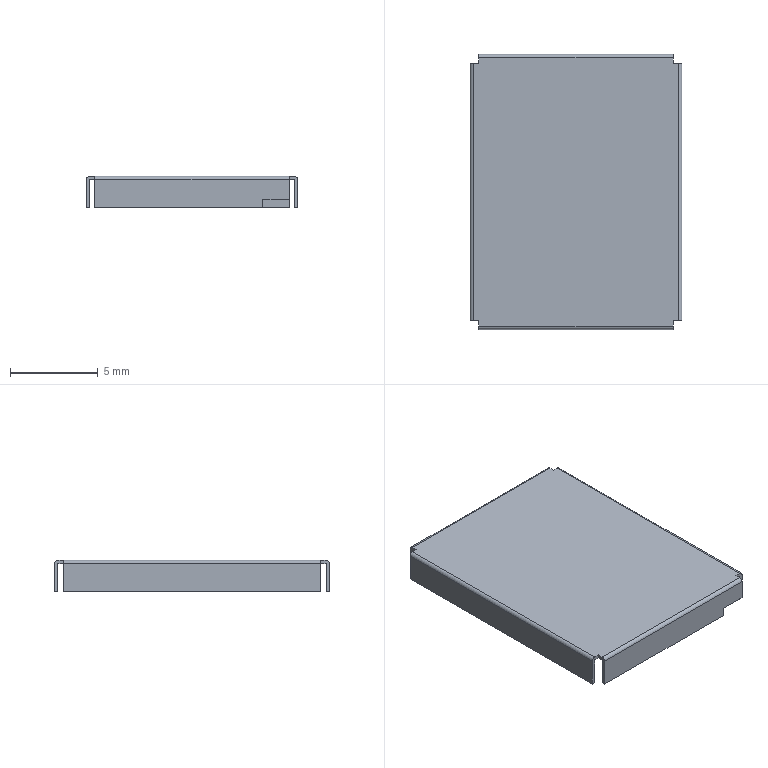Part | Creo | 1 solid | 28 faces | box 12.1 x 15.71 x 1.8 mm | volume 53.743 mm3 | plane 24 | cylinder 4 | commonest cylinder face diameters 0.4 x4
STEP:
#1=CARTESIAN_POINT('',(0.,0.,0.));
#2=DIRECTION('',(0.,0.,1.));
#3=DIRECTION('',(1.,0.,0.));
#4=AXIS2_PLACEMENT_3D('',#1,#2,#3);
#5=CARTESIAN_POINT('',(-0.1,15.11,0.));
#6=VERTEX_POINT('',#5);
#7=CARTESIAN_POINT('',(0.1,15.11,0.));
#8=VERTEX_POINT('',#7);
#9=CARTESIAN_POINT('',(-0.1,15.11,0.));
#10=DIRECTION('',(1.,0.,0.));
#11=VECTOR('',#10,0.2);
#12=LINE('',#9,#11);
#13=EDGE_CURVE('',#6,#8,#12,.T.);
#14=ORIENTED_EDGE('',*,*,#13,.F.);
#15=CARTESIAN_POINT('',(-0.1,0.4,0.));
#16=VERTEX_POINT('',#15);
#17=CARTESIAN_POINT('',(-0.1,15.11,0.));
#18=DIRECTION('',(0.,-1.,0.));
#19=VECTOR('',#18,14.71);
#20=LINE('',#17,#19);
#21=EDGE_CURVE('',#6,#16,#20,.T.);
#22=ORIENTED_EDGE('',*,*,#21,.T.);
#23=CARTESIAN_POINT('',(0.1,0.4,0.));
#24=VERTEX_POINT('',#23);
#25=CARTESIAN_POINT('',(-0.1,0.4,0.));
#26=DIRECTION('',(1.,0.,0.));
#27=VECTOR('',#26,0.2);
#28=LINE('',#25,#27);
#29=EDGE_CURVE('',#16,#24,#28,.T.);
#30=ORIENTED_EDGE('',*,*,#29,.T.);
#31=CARTESIAN_POINT('',(0.1,15.11,0.));
#32=DIRECTION('',(0.,-1.,0.));
#33=VECTOR('',#32,14.71);
#34=LINE('',#31,#33);
#35=EDGE_CURVE('',#8,#24,#34,.T.);
#36=ORIENTED_EDGE('',*,*,#35,.F.);
#37=EDGE_LOOP('',(#14,#22,#30,#36));
#38=FACE_OUTER_BOUND('',#37,.F.);
#39=CARTESIAN_POINT('',(0.,0.,0.));
#40=DIRECTION('',(0.,0.,1.));
#41=DIRECTION('',(1.,0.,0.));
#42=AXIS2_PLACEMENT_3D('',#39,#40,#41);
#43=PLANE('',#42);
#44=ADVANCED_FACE('',(#38),#43,.F.);
#45=ORIENTED_EDGE('',*,*,#13,.T.);
#46=CARTESIAN_POINT('',(0.1,15.11,1.6));
#47=VERTEX_POINT('',#46);
#48=CARTESIAN_POINT('',(0.1,15.11,0.));
#49=DIRECTION('',(0.,0.,1.));
#50=VECTOR('',#49,1.6);
#51=LINE('',#48,#50);
#52=EDGE_CURVE('',#8,#47,#51,.T.);
#53=ORIENTED_EDGE('',*,*,#52,.T.);
#54=CARTESIAN_POINT('',(0.4,15.11,1.6));
#55=VERTEX_POINT('',#54);
#56=CARTESIAN_POINT('',(0.1,15.11,1.6));
#57=DIRECTION('',(1.,0.,0.));
#58=VECTOR('',#57,0.3);
#59=LINE('',#56,#58);
#60=EDGE_CURVE('',#47,#55,#59,.T.);
#61=ORIENTED_EDGE('',*,*,#60,.T.);
#62=CARTESIAN_POINT('',(0.4,15.11,1.8));
#63=VERTEX_POINT('',#62);
#64=CARTESIAN_POINT('',(0.4,15.11,1.8));
#65=DIRECTION('',(0.,0.,-1.));
#66=VECTOR('',#65,0.2);
#67=LINE('',#64,#66);
#68=EDGE_CURVE('',#63,#55,#67,.T.);
#69=ORIENTED_EDGE('',*,*,#68,.F.);
#70=CARTESIAN_POINT('',(0.1,15.11,1.8));
#71=VERTEX_POINT('',#70);
#72=CARTESIAN_POINT('',(0.1,15.11,1.8));
#73=DIRECTION('',(1.,0.,0.));
#74=VECTOR('',#73,0.3);
#75=LINE('',#72,#74);
#76=EDGE_CURVE('',#71,#63,#75,.T.);
#77=ORIENTED_EDGE('',*,*,#76,.F.);
#78=CARTESIAN_POINT('',(-0.1,15.11,1.6));
#79=VERTEX_POINT('',#78);
#80=CARTESIAN_POINT('',(0.1,15.11,1.6));
#81=DIRECTION('',(0.,-1.,0.));
#82=DIRECTION('',(0.,0.,1.));
#83=AXIS2_PLACEMENT_3D('',#80,#81,#82);
#84=CIRCLE('',#83,0.2);
#85=EDGE_CURVE('',#71,#79,#84,.T.);
#86=ORIENTED_EDGE('',*,*,#85,.T.);
#87=CARTESIAN_POINT('',(-0.1,15.11,0.));
#88=DIRECTION('',(0.,0.,1.));
#89=VECTOR('',#88,1.6);
#90=LINE('',#87,#89);
#91=EDGE_CURVE('',#6,#79,#90,.T.);
#92=ORIENTED_EDGE('',*,*,#91,.F.);
#93=EDGE_LOOP('',(#45,#53,#61,#69,#77,#86,#92));
#94=FACE_OUTER_BOUND('',#93,.F.);
#95=CARTESIAN_POINT('',(-0.1,15.11,1.8));
#96=DIRECTION('',(0.,-1.,0.));
#97=DIRECTION('',(1.,0.,0.));
#98=AXIS2_PLACEMENT_3D('',#95,#96,#97);
#99=PLANE('',#98);
#100=ADVANCED_FACE('',(#94),#99,.F.);
#101=ORIENTED_EDGE('',*,*,#52,.F.);
#102=ORIENTED_EDGE('',*,*,#35,.T.);
#103=CARTESIAN_POINT('',(0.1,0.4,1.6));
#104=VERTEX_POINT('',#103);
#105=CARTESIAN_POINT('',(0.1,0.4,0.));
#106=DIRECTION('',(0.,0.,1.));
#107=VECTOR('',#106,1.6);
#108=LINE('',#105,#107);
#109=EDGE_CURVE('',#24,#104,#108,.T.);
#110=ORIENTED_EDGE('',*,*,#109,.T.);
#111=CARTESIAN_POINT('',(0.1,15.11,1.6));
#112=DIRECTION('',(0.,-1.,0.));
#113=VECTOR('',#112,14.71);
#114=LINE('',#111,#113);
#115=EDGE_CURVE('',#47,#104,#114,.T.);
#116=ORIENTED_EDGE('',*,*,#115,.F.);
#117=EDGE_LOOP('',(#101,#102,#110,#116));
#118=FACE_OUTER_BOUND('',#117,.F.);
#119=CARTESIAN_POINT('',(0.1,15.61,0.));
#120=DIRECTION('',(-1.,0.,0.));
#121=DIRECTION('',(0.,-1.,0.));
#122=AXIS2_PLACEMENT_3D('',#119,#120,#121);
#123=PLANE('',#122);
#124=ADVANCED_FACE('',(#118),#123,.F.);
#125=ORIENTED_EDGE('',*,*,#29,.F.);
#126=CARTESIAN_POINT('',(-0.1,0.4,1.6));
#127=VERTEX_POINT('',#126);
#128=CARTESIAN_POINT('',(-0.1,0.4,0.));
#129=DIRECTION('',(0.,0.,1.));
#130=VECTOR('',#129,1.6);
#131=LINE('',#128,#130);
#132=EDGE_CURVE('',#16,#127,#131,.T.);
#133=ORIENTED_EDGE('',*,*,#132,.T.);
#134=CARTESIAN_POINT('',(0.1,0.4,1.8));
#135=VERTEX_POINT('',#134);
#136=CARTESIAN_POINT('',(0.1,0.4,1.6));
#137=DIRECTION('',(0.,1.,0.));
#138=DIRECTION('',(-1.,0.,0.));
#139=AXIS2_PLACEMENT_3D('',#136,#137,#138);
#140=CIRCLE('',#139,0.2);
#141=EDGE_CURVE('',#127,#135,#140,.T.);
#142=ORIENTED_EDGE('',*,*,#141,.T.);
#143=CARTESIAN_POINT('',(0.4,0.4,1.8));
#144=VERTEX_POINT('',#143);
#145=CARTESIAN_POINT('',(0.1,0.4,1.8));
#146=DIRECTION('',(1.,0.,0.));
#147=VECTOR('',#146,0.3);
#148=LINE('',#145,#147);
#149=EDGE_CURVE('',#135,#144,#148,.T.);
#150=ORIENTED_EDGE('',*,*,#149,.T.);
#151=CARTESIAN_POINT('',(0.4,0.4,1.6));
#152=VERTEX_POINT('',#151);
#153=CARTESIAN_POINT('',(0.4,0.4,1.8));
#154=DIRECTION('',(0.,0.,-1.));
#155=VECTOR('',#154,0.2);
#156=LINE('',#153,#155);
#157=EDGE_CURVE('',#144,#152,#156,.T.);
#158=ORIENTED_EDGE('',*,*,#157,.T.);
#159=CARTESIAN_POINT('',(0.1,0.4,1.6));
#160=DIRECTION('',(1.,0.,0.));
#161=VECTOR('',#160,0.3);
#162=LINE('',#159,#161);
#163=EDGE_CURVE('',#104,#152,#162,.T.);
#164=ORIENTED_EDGE('',*,*,#163,.F.);
#165=ORIENTED_EDGE('',*,*,#109,.F.);
#166=EDGE_LOOP('',(#125,#133,#142,#150,#158,#164,#165));
#167=FACE_OUTER_BOUND('',#166,.F.);
#168=CARTESIAN_POINT('',(0.4,0.4,1.8));
#169=DIRECTION('',(0.,1.,0.));
#170=DIRECTION('',(-1.,0.,0.));
#171=AXIS2_PLACEMENT_3D('',#168,#169,#170);
#172=PLANE('',#171);
#173=ADVANCED_FACE('',(#167),#172,.F.);
#174=ORIENTED_EDGE('',*,*,#91,.T.);
#175=CARTESIAN_POINT('',(-0.1,0.4,1.6));
#176=DIRECTION('',(0.,1.,0.));
#177=VECTOR('',#176,14.71);
#178=LINE('',#175,#177);
#179=EDGE_CURVE('',#127,#79,#178,.T.);
#180=ORIENTED_EDGE('',*,*,#179,.F.);
#181=ORIENTED_EDGE('',*,*,#132,.F.);
#182=ORIENTED_EDGE('',*,*,#21,.F.);
#183=EDGE_LOOP('',(#174,#180,#181,#182));
#184=FACE_OUTER_BOUND('',#183,.F.);
#185=CARTESIAN_POINT('',(-0.1,15.61,0.));
#186=DIRECTION('',(-1.,0.,0.));
#187=DIRECTION('',(0.,-1.,0.));
#188=AXIS2_PLACEMENT_3D('',#185,#186,#187);
#189=PLANE('',#188);
#190=ADVANCED_FACE('',(#184),#189,.T.);
#191=ORIENTED_EDGE('',*,*,#85,.F.);
#192=CARTESIAN_POINT('',(0.1,15.11,1.8));
#193=DIRECTION('',(0.,-1.,0.));
#194=VECTOR('',#193,14.71);
#195=LINE('',#192,#194);
#196=EDGE_CURVE('',#71,#135,#195,.T.);
#197=ORIENTED_EDGE('',*,*,#196,.T.);
#198=ORIENTED_EDGE('',*,*,#141,.F.);
#199=ORIENTED_EDGE('',*,*,#179,.T.);
#200=EDGE_LOOP('',(#191,#197,#198,#199));
#201=FACE_OUTER_BOUND('',#200,.F.);
#202=CARTESIAN_POINT('',(0.1,36.247,1.6));
#203=DIRECTION('',(0.,-1.,0.));
#204=DIRECTION('',(0.,0.,1.));
#205=AXIS2_PLACEMENT_3D('',#202,#203,#204);
#206=CYLINDRICAL_SURFACE('',#205,0.2);
#207=ADVANCED_FACE('',(#201),#206,.T.);
#208=ORIENTED_EDGE('',*,*,#76,.T.);
#209=CARTESIAN_POINT('',(0.4,15.41,1.8));
#210=VERTEX_POINT('',#209);
#211=CARTESIAN_POINT('',(0.4,15.41,1.8));
#212=DIRECTION('',(0.,-1.,0.));
#213=VECTOR('',#212,0.3);
#214=LINE('',#211,#213);
#215=EDGE_CURVE('',#210,#63,#214,.T.);
#216=ORIENTED_EDGE('',*,*,#215,.F.);
#217=CARTESIAN_POINT('',(11.5,15.41,1.8));
#218=VERTEX_POINT('',#217);
#219=CARTESIAN_POINT('',(11.5,15.41,1.8));
#220=DIRECTION('',(-1.,0.,0.));
#221=VECTOR('',#220,11.1);
#222=LINE('',#219,#221);
#223=EDGE_CURVE('',#218,#210,#222,.T.);
#224=ORIENTED_EDGE('',*,*,#223,.F.);
#225=CARTESIAN_POINT('',(11.5,15.11,1.8));
#226=VERTEX_POINT('',#225);
#227=CARTESIAN_POINT('',(11.5,15.41,1.8));
#228=DIRECTION('',(0.,-1.,0.));
#229=VECTOR('',#228,0.3);
#230=LINE('',#227,#229);
#231=EDGE_CURVE('',#218,#226,#230,.T.);
#232=ORIENTED_EDGE('',*,*,#231,.T.);
#233=CARTESIAN_POINT('',(11.8,15.11,1.8));
#234=VERTEX_POINT('',#233);
#235=CARTESIAN_POINT('',(11.8,15.11,1.8));
#236=DIRECTION('',(-1.,0.,0.));
#237=VECTOR('',#236,0.3);
#238=LINE('',#235,#237);
#239=EDGE_CURVE('',#234,#226,#238,.T.);
#240=ORIENTED_EDGE('',*,*,#239,.F.);
#241=CARTESIAN_POINT('',(11.8,0.4,1.8));
#242=VERTEX_POINT('',#241);
#243=CARTESIAN_POINT('',(11.8,0.4,1.8));
#244=DIRECTION('',(0.,1.,0.));
#245=VECTOR('',#244,14.71);
#246=LINE('',#243,#245);
#247=EDGE_CURVE('',#242,#234,#246,.T.);
#248=ORIENTED_EDGE('',*,*,#247,.F.);
#249=CARTESIAN_POINT('',(11.5,0.4,1.8));
#250=VERTEX_POINT('',#249);
#251=CARTESIAN_POINT('',(11.8,0.4,1.8));
#252=DIRECTION('',(-1.,0.,0.));
#253=VECTOR('',#252,0.3);
#254=LINE('',#251,#253);
#255=EDGE_CURVE('',#242,#250,#254,.T.);
#256=ORIENTED_EDGE('',*,*,#255,.T.);
#257=CARTESIAN_POINT('',(11.5,0.1,1.8));
#258=VERTEX_POINT('',#257);
#259=CARTESIAN_POINT('',(11.5,0.1,1.8));
#260=DIRECTION('',(0.,1.,0.));
#261=VECTOR('',#260,0.3);
#262=LINE('',#259,#261);
#263=EDGE_CURVE('',#258,#250,#262,.T.);
#264=ORIENTED_EDGE('',*,*,#263,.F.);
#265=CARTESIAN_POINT('',(0.4,0.1,1.8));
#266=VERTEX_POINT('',#265);
#267=CARTESIAN_POINT('',(0.4,0.1,1.8));
#268=DIRECTION('',(1.,0.,0.));
#269=VECTOR('',#268,11.1);
#270=LINE('',#267,#269);
#271=EDGE_CURVE('',#266,#258,#270,.T.);
#272=ORIENTED_EDGE('',*,*,#271,.F.);
#273=CARTESIAN_POINT('',(0.4,0.1,1.8));
#274=DIRECTION('',(0.,1.,0.));
#275=VECTOR('',#274,0.3);
#276=LINE('',#273,#275);
#277=EDGE_CURVE('',#266,#144,#276,.T.);
#278=ORIENTED_EDGE('',*,*,#277,.T.);
#279=ORIENTED_EDGE('',*,*,#149,.F.);
#280=ORIENTED_EDGE('',*,*,#196,.F.);
#281=EDGE_LOOP('',(#208,#216,#224,#232,#240,#248,#256,#264,#272,#278,#279,#280));
#282=FACE_OUTER_BOUND('',#281,.F.);
#283=CARTESIAN_POINT('',(0.,0.,1.8));
#284=DIRECTION('',(0.,0.,1.));
#285=DIRECTION('',(1.,0.,0.));
#286=AXIS2_PLACEMENT_3D('',#283,#284,#285);
#287=PLANE('',#286);
#288=ADVANCED_FACE('',(#282),#287,.T.);
#289=CARTESIAN_POINT('',(0.4,15.61,0.));
#290=VERTEX_POINT('',#289);
#291=CARTESIAN_POINT('',(0.4,15.41,0.));
#292=VERTEX_POINT('',#291);
#293=CARTESIAN_POINT('',(0.4,15.61,0.));
#294=DIRECTION('',(0.,-1.,0.));
#295=VECTOR('',#294,0.2);
#296=LINE('',#293,#295);
#297=EDGE_CURVE('',#290,#292,#296,.T.);
#298=ORIENTED_EDGE('',*,*,#297,.F.);
#299=CARTESIAN_POINT('',(0.4,15.61,1.6));
#300=VERTEX_POINT('',#299);
#301=CARTESIAN_POINT('',(0.4,15.61,0.));
#302=DIRECTION('',(0.,0.,1.));
#303=VECTOR('',#302,1.6);
#304=LINE('',#301,#303);
#305=EDGE_CURVE('',#290,#300,#304,.T.);
#306=ORIENTED_EDGE('',*,*,#305,.T.);
#307=CARTESIAN_POINT('',(0.4,15.41,1.6));
#308=DIRECTION('',(1.,0.,0.));
#309=DIRECTION('',(0.,1.,0.));
#310=AXIS2_PLACEMENT_3D('',#307,#308,#309);
#311=CIRCLE('',#310,0.2);
#312=EDGE_CURVE('',#300,#210,#311,.T.);
#313=ORIENTED_EDGE('',*,*,#312,.T.);
#314=ORIENTED_EDGE('',*,*,#215,.T.);
#315=ORIENTED_EDGE('',*,*,#68,.T.);
#316=CARTESIAN_POINT('',(0.4,15.41,1.6));
#317=VERTEX_POINT('',#316);
#318=CARTESIAN_POINT('',(0.4,15.41,1.6));
#319=DIRECTION('',(0.,-1.,0.));
#320=VECTOR('',#319,0.3);
#321=LINE('',#318,#320);
#322=EDGE_CURVE('',#317,#55,#321,.T.);
#323=ORIENTED_EDGE('',*,*,#322,.F.);
#324=CARTESIAN_POINT('',(0.4,15.41,0.));
#325=DIRECTION('',(0.,0.,1.));
#326=VECTOR('',#325,1.6);
#327=LINE('',#324,#326);
#328=EDGE_CURVE('',#292,#317,#327,.T.);
#329=ORIENTED_EDGE('',*,*,#328,.F.);
#330=EDGE_LOOP('',(#298,#306,#313,#314,#315,#323,#329));
#331=FACE_OUTER_BOUND('',#330,.F.);
#332=CARTESIAN_POINT('',(0.4,15.11,1.8));
#333=DIRECTION('',(1.,0.,0.));
#334=DIRECTION('',(0.,1.,0.));
#335=AXIS2_PLACEMENT_3D('',#332,#333,#334);
#336=PLANE('',#335);
#337=ADVANCED_FACE('',(#331),#336,.F.);
#338=ORIENTED_EDGE('',*,*,#297,.T.);
#339=CARTESIAN_POINT('',(11.5,15.41,0.));
#340=VERTEX_POINT('',#339);
#341=CARTESIAN_POINT('',(11.5,15.41,0.));
#342=DIRECTION('',(-1.,0.,0.));
#343=VECTOR('',#342,11.1);
#344=LINE('',#341,#343);
#345=EDGE_CURVE('',#340,#292,#344,.T.);
#346=ORIENTED_EDGE('',*,*,#345,.F.);
#347=CARTESIAN_POINT('',(11.5,15.61,0.));
#348=VERTEX_POINT('',#347);
#349=CARTESIAN_POINT('',(11.5,15.61,0.));
#350=DIRECTION('',(0.,-1.,0.));
#351=VECTOR('',#350,0.2);
#352=LINE('',#349,#351);
#353=EDGE_CURVE('',#348,#340,#352,.T.);
#354=ORIENTED_EDGE('',*,*,#353,.F.);
#355=CARTESIAN_POINT('',(11.5,15.61,0.));
#356=DIRECTION('',(-1.,0.,0.));
#357=VECTOR('',#356,11.1);
#358=LINE('',#355,#357);
#359=EDGE_CURVE('',#348,#290,#358,.T.);
#360=ORIENTED_EDGE('',*,*,#359,.T.);
#361=EDGE_LOOP('',(#338,#346,#354,#360));
#362=FACE_OUTER_BOUND('',#361,.F.);
#363=CARTESIAN_POINT('',(0.,0.,0.));
#364=DIRECTION('',(0.,0.,1.));
#365=DIRECTION('',(1.,0.,0.));
#366=AXIS2_PLACEMENT_3D('',#363,#364,#365);
#367=PLANE('',#366);
#368=ADVANCED_FACE('',(#362),#367,.F.);
#369=ORIENTED_EDGE('',*,*,#328,.T.);
#370=CARTESIAN_POINT('',(11.5,15.41,1.6));
#371=VERTEX_POINT('',#370);
#372=CARTESIAN_POINT('',(11.5,15.41,1.6));
#373=DIRECTION('',(-1.,0.,0.));
#374=VECTOR('',#373,11.1);
#375=LINE('',#372,#374);
#376=EDGE_CURVE('',#371,#317,#375,.T.);
#377=ORIENTED_EDGE('',*,*,#376,.F.);
#378=CARTESIAN_POINT('',(11.5,15.41,0.));
#379=DIRECTION('',(0.,0.,1.));
#380=VECTOR('',#379,1.6);
#381=LINE('',#378,#380);
#382=EDGE_CURVE('',#340,#371,#381,.T.);
#383=ORIENTED_EDGE('',*,*,#382,.F.);
#384=ORIENTED_EDGE('',*,*,#345,.T.);
#385=EDGE_LOOP('',(#369,#377,#383,#384));
#386=FACE_OUTER_BOUND('',#385,.F.);
#387=CARTESIAN_POINT('',(12.,15.41,0.));
#388=DIRECTION('',(0.,1.,0.));
#389=DIRECTION('',(-1.,0.,0.));
#390=AXIS2_PLACEMENT_3D('',#387,#388,#389);
#391=PLANE('',#390);
#392=ADVANCED_FACE('',(#386),#391,.F.);
#393=ORIENTED_EDGE('',*,*,#60,.F.);
#394=ORIENTED_EDGE('',*,*,#115,.T.);
#395=ORIENTED_EDGE('',*,*,#163,.T.);
#396=CARTESIAN_POINT('',(0.4,0.1,1.6));
#397=VERTEX_POINT('',#396);
#398=CARTESIAN_POINT('',(0.4,0.1,1.6));
#399=DIRECTION('',(0.,1.,0.));
#400=VECTOR('',#399,0.3);
#401=LINE('',#398,#400);
#402=EDGE_CURVE('',#397,#152,#401,.T.);
#403=ORIENTED_EDGE('',*,*,#402,.F.);
#404=CARTESIAN_POINT('',(11.5,0.1,1.6));
#405=VERTEX_POINT('',#404);
#406=CARTESIAN_POINT('',(0.4,0.1,1.6));
#407=DIRECTION('',(1.,0.,0.));
#408=VECTOR('',#407,11.1);
#409=LINE('',#406,#408);
#410=EDGE_CURVE('',#397,#405,#409,.T.);
#411=ORIENTED_EDGE('',*,*,#410,.T.);
#412=CARTESIAN_POINT('',(11.5,0.4,1.6));
#413=VERTEX_POINT('',#412);
#414=CARTESIAN_POINT('',(11.5,0.1,1.6));
#415=DIRECTION('',(0.,1.,0.));
#416=VECTOR('',#415,0.3);
#417=LINE('',#414,#416);
#418=EDGE_CURVE('',#405,#413,#417,.T.);
#419=ORIENTED_EDGE('',*,*,#418,.T.);
#420=CARTESIAN_POINT('',(11.8,0.4,1.6));
#421=VERTEX_POINT('',#420);
#422=CARTESIAN_POINT('',(11.8,0.4,1.6));
#423=DIRECTION('',(-1.,0.,0.));
#424=VECTOR('',#423,0.3);
#425=LINE('',#422,#424);
#426=EDGE_CURVE('',#421,#413,#425,.T.);
#427=ORIENTED_EDGE('',*,*,#426,.F.);
#428=CARTESIAN_POINT('',(11.8,15.11,1.6));
#429=VERTEX_POINT('',#428);
#430=CARTESIAN_POINT('',(11.8,0.4,1.6));
#431=DIRECTION('',(0.,1.,0.));
#432=VECTOR('',#431,14.71);
#433=LINE('',#430,#432);
#434=EDGE_CURVE('',#421,#429,#433,.T.);
#435=ORIENTED_EDGE('',*,*,#434,.T.);
#436=CARTESIAN_POINT('',(11.5,15.11,1.6));
#437=VERTEX_POINT('',#436);
#438=CARTESIAN_POINT('',(11.8,15.11,1.6));
#439=DIRECTION('',(-1.,0.,0.));
#440=VECTOR('',#439,0.3);
#441=LINE('',#438,#440);
#442=EDGE_CURVE('',#429,#437,#441,.T.);
#443=ORIENTED_EDGE('',*,*,#442,.T.);
#444=CARTESIAN_POINT('',(11.5,15.41,1.6));
#445=DIRECTION('',(0.,-1.,0.));
#446=VECTOR('',#445,0.3);
#447=LINE('',#444,#446);
#448=EDGE_CURVE('',#371,#437,#447,.T.);
#449=ORIENTED_EDGE('',*,*,#448,.F.);
#450=ORIENTED_EDGE('',*,*,#376,.T.);
#451=ORIENTED_EDGE('',*,*,#322,.T.);
#452=EDGE_LOOP('',(#393,#394,#395,#403,#411,#419,#427,#435,#443,#449,#450,#451));
#453=FACE_OUTER_BOUND('',#452,.F.);
#454=CARTESIAN_POINT('',(0.,0.,1.6));
#455=DIRECTION('',(0.,0.,1.));
#456=DIRECTION('',(1.,0.,0.));
#457=AXIS2_PLACEMENT_3D('',#454,#455,#456);
#458=PLANE('',#457);
#459=ADVANCED_FACE('',(#453),#458,.F.);
#460=CARTESIAN_POINT('',(0.4,-0.1,0.));
#461=VERTEX_POINT('',#460);
#462=CARTESIAN_POINT('',(0.4,0.1,0.));
#463=VERTEX_POINT('',#462);
#464=CARTESIAN_POINT('',(0.4,-0.1,0.));
#465=DIRECTION('',(0.,1.,0.));
#466=VECTOR('',#465,0.2);
#467=LINE('',#464,#466);
#468=EDGE_CURVE('',#461,#463,#467,.T.);
#469=ORIENTED_EDGE('',*,*,#468,.T.);
#470=CARTESIAN_POINT('',(0.4,0.1,0.));
#471=DIRECTION('',(0.,0.,1.));
#472=VECTOR('',#471,1.6);
#473=LINE('',#470,#472);
#474=EDGE_CURVE('',#463,#397,#473,.T.);
#475=ORIENTED_EDGE('',*,*,#474,.T.);
#476=ORIENTED_EDGE('',*,*,#402,.T.);
#477=ORIENTED_EDGE('',*,*,#157,.F.);
#478=ORIENTED_EDGE('',*,*,#277,.F.);
#479=CARTESIAN_POINT('',(0.4,-0.1,1.6));
#480=VERTEX_POINT('',#479);
#481=CARTESIAN_POINT('',(0.4,0.1,1.6));
#482=DIRECTION('',(1.,0.,0.));
#483=DIRECTION('',(0.,0.,1.));
#484=AXIS2_PLACEMENT_3D('',#481,#482,#483);
#485=CIRCLE('',#484,0.2);
#486=EDGE_CURVE('',#266,#480,#485,.T.);
#487=ORIENTED_EDGE('',*,*,#486,.T.);
#488=CARTESIAN_POINT('',(0.4,-0.1,0.));
#489=DIRECTION('',(0.,0.,1.));
#490=VECTOR('',#489,1.6);
#491=LINE('',#488,#490);
#492=EDGE_CURVE('',#461,#480,#491,.T.);
#493=ORIENTED_EDGE('',*,*,#492,.F.);
#494=EDGE_LOOP('',(#469,#475,#476,#477,#478,#487,#493));
#495=FACE_OUTER_BOUND('',#494,.F.);
#496=CARTESIAN_POINT('',(0.4,-0.1,1.8));
#497=DIRECTION('',(1.,0.,0.));
#498=DIRECTION('',(0.,1.,0.));
#499=AXIS2_PLACEMENT_3D('',#496,#497,#498);
#500=PLANE('',#499);
#501=ADVANCED_FACE('',(#495),#500,.F.);
#502=CARTESIAN_POINT('',(10.,-0.1,0.));
#503=VERTEX_POINT('',#502);
#504=CARTESIAN_POINT('',(10.,0.1,0.));
#505=VERTEX_POINT('',#504);
#506=CARTESIAN_POINT('',(10.,-0.1,0.));
#507=DIRECTION('',(0.,1.,0.));
#508=VECTOR('',#507,0.2);
#509=LINE('',#506,#508);
#510=EDGE_CURVE('',#503,#505,#509,.T.);
#511=ORIENTED_EDGE('',*,*,#510,.T.);
#512=CARTESIAN_POINT('',(0.4,0.1,0.));
#513=DIRECTION('',(1.,0.,0.));
#514=VECTOR('',#513,9.6);
#515=LINE('',#512,#514);
#516=EDGE_CURVE('',#463,#505,#515,.T.);
#517=ORIENTED_EDGE('',*,*,#516,.F.);
#518=ORIENTED_EDGE('',*,*,#468,.F.);
#519=CARTESIAN_POINT('',(0.4,-0.1,0.));
#520=DIRECTION('',(1.,0.,0.));
#521=VECTOR('',#520,9.6);
#522=LINE('',#519,#521);
#523=EDGE_CURVE('',#461,#503,#522,.T.);
#524=ORIENTED_EDGE('',*,*,#523,.T.);
#525=EDGE_LOOP('',(#511,#517,#518,#524));
#526=FACE_OUTER_BOUND('',#525,.F.);
#527=CARTESIAN_POINT('',(0.,0.,0.));
#528=DIRECTION('',(0.,0.,1.));
#529=DIRECTION('',(1.,0.,0.));
#530=AXIS2_PLACEMENT_3D('',#527,#528,#529);
#531=PLANE('',#530);
#532=ADVANCED_FACE('',(#526),#531,.F.);
#533=ORIENTED_EDGE('',*,*,#510,.F.);
#534=CARTESIAN_POINT('',(10.,-0.1,0.5));
#535=VERTEX_POINT('',#534);
#536=CARTESIAN_POINT('',(10.,-0.1,0.));
#537=DIRECTION('',(0.,0.,1.));
#538=VECTOR('',#537,0.5);
#539=LINE('',#536,#538);
#540=EDGE_CURVE('',#503,#535,#539,.T.);
#541=ORIENTED_EDGE('',*,*,#540,.T.);
#542=CARTESIAN_POINT('',(10.,0.1,0.5));
#543=VERTEX_POINT('',#542);
#544=CARTESIAN_POINT('',(10.,-0.1,0.5));
#545=DIRECTION('',(0.,1.,0.));
#546=VECTOR('',#545,0.2);
#547=LINE('',#544,#546);
#548=EDGE_CURVE('',#535,#543,#547,.T.);
#549=ORIENTED_EDGE('',*,*,#548,.T.);
#550=CARTESIAN_POINT('',(10.,0.1,0.));
#551=DIRECTION('',(0.,0.,1.));
#552=VECTOR('',#551,0.5);
#553=LINE('',#550,#552);
#554=EDGE_CURVE('',#505,#543,#553,.T.);
#555=ORIENTED_EDGE('',*,*,#554,.F.);
#556=EDGE_LOOP('',(#533,#541,#549,#555));
#557=FACE_OUTER_BOUND('',#556,.F.);
#558=CARTESIAN_POINT('',(10.,-0.1,0.));
#559=DIRECTION('',(-1.,0.,0.));
#560=DIRECTION('',(0.,1.,0.));
#561=AXIS2_PLACEMENT_3D('',#558,#559,#560);
#562=PLANE('',#561);
#563=ADVANCED_FACE('',(#557),#562,.F.);
#564=CARTESIAN_POINT('',(11.5,-0.1,0.5));
#565=VERTEX_POINT('',#564);
#566=CARTESIAN_POINT('',(11.5,-0.1,0.5));
#567=DIRECTION('',(-1.,0.,0.));
#568=VECTOR('',#567,1.5);
#569=LINE('',#566,#568);
#570=EDGE_CURVE('',#565,#535,#569,.T.);
#571=ORIENTED_EDGE('',*,*,#570,.T.);
#572=ORIENTED_EDGE('',*,*,#540,.F.);
#573=ORIENTED_EDGE('',*,*,#523,.F.);
#574=ORIENTED_EDGE('',*,*,#492,.T.);
#575=CARTESIAN_POINT('',(11.5,-0.1,1.6));
#576=VERTEX_POINT('',#575);
#577=CARTESIAN_POINT('',(11.5,-0.1,1.6));
#578=DIRECTION('',(-1.,0.,0.));
#579=VECTOR('',#578,11.1);
#580=LINE('',#577,#579);
#581=EDGE_CURVE('',#576,#480,#580,.T.);
#582=ORIENTED_EDGE('',*,*,#581,.F.);
#583=CARTESIAN_POINT('',(11.5,-0.1,0.5));
#584=DIRECTION('',(0.,0.,1.));
#585=VECTOR('',#584,1.1);
#586=LINE('',#583,#585);
#587=EDGE_CURVE('',#565,#576,#586,.T.);
#588=ORIENTED_EDGE('',*,*,#587,.F.);
#589=EDGE_LOOP('',(#571,#572,#573,#574,#582,#588));
#590=FACE_OUTER_BOUND('',#589,.F.);
#591=CARTESIAN_POINT('',(-0.1,-0.1,0.));
#592=DIRECTION('',(0.,-1.,0.));
#593=DIRECTION('',(1.,0.,0.));
#594=AXIS2_PLACEMENT_3D('',#591,#592,#593);
#595=PLANE('',#594);
#596=ADVANCED_FACE('',(#590),#595,.T.);
#597=ORIENTED_EDGE('',*,*,#570,.F.);
#598=CARTESIAN_POINT('',(11.5,0.1,0.5));
#599=VERTEX_POINT('',#598);
#600=CARTESIAN_POINT('',(11.5,-0.1,0.5));
#601=DIRECTION('',(0.,1.,0.));
#602=VECTOR('',#601,0.2);
#603=LINE('',#600,#602);
#604=EDGE_CURVE('',#565,#599,#603,.T.);
#605=ORIENTED_EDGE('',*,*,#604,.T.);
#606=CARTESIAN_POINT('',(11.5,0.1,0.5));
#607=DIRECTION('',(-1.,0.,0.));
#608=VECTOR('',#607,1.5);
#609=LINE('',#606,#608);
#610=EDGE_CURVE('',#599,#543,#609,.T.);
#611=ORIENTED_EDGE('',*,*,#610,.T.);
#612=ORIENTED_EDGE('',*,*,#548,.F.);
#613=EDGE_LOOP('',(#597,#605,#611,#612));
#614=FACE_OUTER_BOUND('',#613,.F.);
#615=CARTESIAN_POINT('',(0.,0.,0.5));
#616=DIRECTION('',(0.,0.,-1.));
#617=DIRECTION('',(1.,0.,0.));
#618=AXIS2_PLACEMENT_3D('',#615,#616,#617);
#619=PLANE('',#618);
#620=ADVANCED_FACE('',(#614),#619,.T.);
#621=ORIENTED_EDGE('',*,*,#604,.F.);
#622=ORIENTED_EDGE('',*,*,#587,.T.);
#623=CARTESIAN_POINT('',(11.5,0.1,1.6));
#624=DIRECTION('',(-1.,0.,0.));
#625=DIRECTION('',(0.,-1.,0.));
#626=AXIS2_PLACEMENT_3D('',#623,#624,#625);
#627=CIRCLE('',#626,0.2);
#628=EDGE_CURVE('',#576,#258,#627,.T.);
#629=ORIENTED_EDGE('',*,*,#628,.T.);
#630=ORIENTED_EDGE('',*,*,#263,.T.);
#631=CARTESIAN_POINT('',(11.5,0.4,1.8));
#632=DIRECTION('',(0.,0.,-1.));
#633=VECTOR('',#632,0.2);
#634=LINE('',#631,#633);
#635=EDGE_CURVE('',#250,#413,#634,.T.);
#636=ORIENTED_EDGE('',*,*,#635,.T.);
#637=ORIENTED_EDGE('',*,*,#418,.F.);
#638=CARTESIAN_POINT('',(11.5,0.1,0.5));
#639=DIRECTION('',(0.,0.,1.));
#640=VECTOR('',#639,1.1);
#641=LINE('',#638,#640);
#642=EDGE_CURVE('',#599,#405,#641,.T.);
#643=ORIENTED_EDGE('',*,*,#642,.F.);
#644=EDGE_LOOP('',(#621,#622,#629,#630,#636,#637,#643));
#645=FACE_OUTER_BOUND('',#644,.F.);
#646=CARTESIAN_POINT('',(11.5,0.4,1.8));
#647=DIRECTION('',(-1.,0.,0.));
#648=DIRECTION('',(0.,-1.,0.));
#649=AXIS2_PLACEMENT_3D('',#646,#647,#648);
#650=PLANE('',#649);
#651=ADVANCED_FACE('',(#645),#650,.F.);
#652=ORIENTED_EDGE('',*,*,#628,.F.);
#653=ORIENTED_EDGE('',*,*,#581,.T.);
#654=ORIENTED_EDGE('',*,*,#486,.F.);
#655=ORIENTED_EDGE('',*,*,#271,.T.);
#656=EDGE_LOOP('',(#652,#653,#654,#655));
#657=FACE_OUTER_BOUND('',#656,.F.);
#658=CARTESIAN_POINT('',(-16.054,0.1,1.6));
#659=DIRECTION('',(1.,0.,0.));
#660=DIRECTION('',(0.,0.,1.));
#661=AXIS2_PLACEMENT_3D('',#658,#659,#660);
#662=CYLINDRICAL_SURFACE('',#661,0.2);
#663=ADVANCED_FACE('',(#657),#662,.T.);
#664=CARTESIAN_POINT('',(12.,0.4,0.));
#665=VERTEX_POINT('',#664);
#666=CARTESIAN_POINT('',(11.8,0.4,0.));
#667=VERTEX_POINT('',#666);
#668=CARTESIAN_POINT('',(12.,0.4,0.));
#669=DIRECTION('',(-1.,0.,0.));
#670=VECTOR('',#669,0.2);
#671=LINE('',#668,#670);
#672=EDGE_CURVE('',#665,#667,#671,.T.);
#673=ORIENTED_EDGE('',*,*,#672,.T.);
#674=CARTESIAN_POINT('',(11.8,0.4,0.));
#675=DIRECTION('',(0.,0.,1.));
#676=VECTOR('',#675,1.6);
#677=LINE('',#674,#676);
#678=EDGE_CURVE('',#667,#421,#677,.T.);
#679=ORIENTED_EDGE('',*,*,#678,.T.);
#680=ORIENTED_EDGE('',*,*,#426,.T.);
#681=ORIENTED_EDGE('',*,*,#635,.F.);
#682=ORIENTED_EDGE('',*,*,#255,.F.);
#683=CARTESIAN_POINT('',(12.,0.4,1.6));
#684=VERTEX_POINT('',#683);
#685=CARTESIAN_POINT('',(11.8,0.4,1.6));
#686=DIRECTION('',(0.,1.,0.));
#687=DIRECTION('',(0.,0.,1.));
#688=AXIS2_PLACEMENT_3D('',#685,#686,#687);
#689=CIRCLE('',#688,0.2);
#690=EDGE_CURVE('',#242,#684,#689,.T.);
#691=ORIENTED_EDGE('',*,*,#690,.T.);
#692=CARTESIAN_POINT('',(12.,0.4,0.));
#693=DIRECTION('',(0.,0.,1.));
#694=VECTOR('',#693,1.6);
#695=LINE('',#692,#694);
#696=EDGE_CURVE('',#665,#684,#695,.T.);
#697=ORIENTED_EDGE('',*,*,#696,.F.);
#698=EDGE_LOOP('',(#673,#679,#680,#681,#682,#691,#697));
#699=FACE_OUTER_BOUND('',#698,.F.);
#700=CARTESIAN_POINT('',(12.,0.4,1.8));
#701=DIRECTION('',(0.,1.,0.));
#702=DIRECTION('',(-1.,0.,0.));
#703=AXIS2_PLACEMENT_3D('',#700,#701,#702);
#704=PLANE('',#703);
#705=ADVANCED_FACE('',(#699),#704,.F.);
#706=CARTESIAN_POINT('',(12.,15.11,0.));
#707=VERTEX_POINT('',#706);
#708=CARTESIAN_POINT('',(11.8,15.11,0.));
#709=VERTEX_POINT('',#708);
#710=CARTESIAN_POINT('',(12.,15.11,0.));
#711=DIRECTION('',(-1.,0.,0.));
#712=VECTOR('',#711,0.2);
#713=LINE('',#710,#712);
#714=EDGE_CURVE('',#707,#709,#713,.T.);
#715=ORIENTED_EDGE('',*,*,#714,.T.);
#716=CARTESIAN_POINT('',(11.8,0.4,0.));
#717=DIRECTION('',(0.,1.,0.));
#718=VECTOR('',#717,14.71);
#719=LINE('',#716,#718);
#720=EDGE_CURVE('',#667,#709,#719,.T.);
#721=ORIENTED_EDGE('',*,*,#720,.F.);
#722=ORIENTED_EDGE('',*,*,#672,.F.);
#723=CARTESIAN_POINT('',(12.,0.4,0.));
#724=DIRECTION('',(0.,1.,0.));
#725=VECTOR('',#724,14.71);
#726=LINE('',#723,#725);
#727=EDGE_CURVE('',#665,#707,#726,.T.);
#728=ORIENTED_EDGE('',*,*,#727,.T.);
#729=EDGE_LOOP('',(#715,#721,#722,#728));
#730=FACE_OUTER_BOUND('',#729,.F.);
#731=CARTESIAN_POINT('',(0.,0.,0.));
#732=DIRECTION('',(0.,0.,1.));
#733=DIRECTION('',(1.,0.,0.));
#734=AXIS2_PLACEMENT_3D('',#731,#732,#733);
#735=PLANE('',#734);
#736=ADVANCED_FACE('',(#730),#735,.F.);
#737=ORIENTED_EDGE('',*,*,#714,.F.);
#738=CARTESIAN_POINT('',(12.,15.11,1.6));
#739=VERTEX_POINT('',#738);
#740=CARTESIAN_POINT('',(12.,15.11,0.));
#741=DIRECTION('',(0.,0.,1.));
#742=VECTOR('',#741,1.6);
#743=LINE('',#740,#742);
#744=EDGE_CURVE('',#707,#739,#743,.T.);
#745=ORIENTED_EDGE('',*,*,#744,.T.);
#746=CARTESIAN_POINT('',(11.8,15.11,1.6));
#747=DIRECTION('',(0.,-1.,0.));
#748=DIRECTION('',(1.,0.,0.));
#749=AXIS2_PLACEMENT_3D('',#746,#747,#748);
#750=CIRCLE('',#749,0.2);
#751=EDGE_CURVE('',#739,#234,#750,.T.);
#752=ORIENTED_EDGE('',*,*,#751,.T.);
#753=ORIENTED_EDGE('',*,*,#239,.T.);
#754=CARTESIAN_POINT('',(11.5,15.11,1.8));
#755=DIRECTION('',(0.,0.,-1.));
#756=VECTOR('',#755,0.2);
#757=LINE('',#754,#756);
#758=EDGE_CURVE('',#226,#437,#757,.T.);
#759=ORIENTED_EDGE('',*,*,#758,.T.);
#760=ORIENTED_EDGE('',*,*,#442,.F.);
#761=CARTESIAN_POINT('',(11.8,15.11,0.));
#762=DIRECTION('',(0.,0.,1.));
#763=VECTOR('',#762,1.6);
#764=LINE('',#761,#763);
#765=EDGE_CURVE('',#709,#429,#764,.T.);
#766=ORIENTED_EDGE('',*,*,#765,.F.);
#767=EDGE_LOOP('',(#737,#745,#752,#753,#759,#760,#766));
#768=FACE_OUTER_BOUND('',#767,.F.);
#769=CARTESIAN_POINT('',(11.5,15.11,1.8));
#770=DIRECTION('',(0.,-1.,0.));
#771=DIRECTION('',(1.,0.,0.));
#772=AXIS2_PLACEMENT_3D('',#769,#770,#771);
#773=PLANE('',#772);
#774=ADVANCED_FACE('',(#768),#773,.F.);
#775=ORIENTED_EDGE('',*,*,#744,.F.);
#776=ORIENTED_EDGE('',*,*,#727,.F.);
#777=ORIENTED_EDGE('',*,*,#696,.T.);
#778=CARTESIAN_POINT('',(12.,15.11,1.6));
#779=DIRECTION('',(0.,-1.,0.));
#780=VECTOR('',#779,14.71);
#781=LINE('',#778,#780);
#782=EDGE_CURVE('',#739,#684,#781,.T.);
#783=ORIENTED_EDGE('',*,*,#782,.F.);
#784=EDGE_LOOP('',(#775,#776,#777,#783));
#785=FACE_OUTER_BOUND('',#784,.F.);
#786=CARTESIAN_POINT('',(12.,-0.1,0.));
#787=DIRECTION('',(1.,0.,0.));
#788=DIRECTION('',(0.,1.,0.));
#789=AXIS2_PLACEMENT_3D('',#786,#787,#788);
#790=PLANE('',#789);
#791=ADVANCED_FACE('',(#785),#790,.T.);
#792=ORIENTED_EDGE('',*,*,#751,.F.);
#793=ORIENTED_EDGE('',*,*,#782,.T.);
#794=ORIENTED_EDGE('',*,*,#690,.F.);
#795=ORIENTED_EDGE('',*,*,#247,.T.);
#796=EDGE_LOOP('',(#792,#793,#794,#795));
#797=FACE_OUTER_BOUND('',#796,.F.);
#798=CARTESIAN_POINT('',(11.8,-20.747,1.6));
#799=DIRECTION('',(0.,1.,0.));
#800=DIRECTION('',(0.,0.,1.));
#801=AXIS2_PLACEMENT_3D('',#798,#799,#800);
#802=CYLINDRICAL_SURFACE('',#801,0.2);
#803=ADVANCED_FACE('',(#797),#802,.T.);
#804=ORIENTED_EDGE('',*,*,#353,.T.);
#805=ORIENTED_EDGE('',*,*,#382,.T.);
#806=ORIENTED_EDGE('',*,*,#448,.T.);
#807=ORIENTED_EDGE('',*,*,#758,.F.);
#808=ORIENTED_EDGE('',*,*,#231,.F.);
#809=CARTESIAN_POINT('',(11.5,15.61,1.6));
#810=VERTEX_POINT('',#809);
#811=CARTESIAN_POINT('',(11.5,15.41,1.6));
#812=DIRECTION('',(-1.,0.,0.));
#813=DIRECTION('',(0.,0.,1.));
#814=AXIS2_PLACEMENT_3D('',#811,#812,#813);
#815=CIRCLE('',#814,0.2);
#816=EDGE_CURVE('',#218,#810,#815,.T.);
#817=ORIENTED_EDGE('',*,*,#816,.T.);
#818=CARTESIAN_POINT('',(11.5,15.61,0.));
#819=DIRECTION('',(0.,0.,1.));
#820=VECTOR('',#819,1.6);
#821=LINE('',#818,#820);
#822=EDGE_CURVE('',#348,#810,#821,.T.);
#823=ORIENTED_EDGE('',*,*,#822,.F.);
#824=EDGE_LOOP('',(#804,#805,#806,#807,#808,#817,#823));
#825=FACE_OUTER_BOUND('',#824,.F.);
#826=CARTESIAN_POINT('',(11.5,15.61,1.8));
#827=DIRECTION('',(-1.,0.,0.));
#828=DIRECTION('',(0.,-1.,0.));
#829=AXIS2_PLACEMENT_3D('',#826,#827,#828);
#830=PLANE('',#829);
#831=ADVANCED_FACE('',(#825),#830,.F.);
#832=ORIENTED_EDGE('',*,*,#312,.F.);
#833=CARTESIAN_POINT('',(0.4,15.61,1.6));
#834=DIRECTION('',(1.,0.,0.));
#835=VECTOR('',#834,11.1);
#836=LINE('',#833,#835);
#837=EDGE_CURVE('',#300,#810,#836,.T.);
#838=ORIENTED_EDGE('',*,*,#837,.T.);
#839=ORIENTED_EDGE('',*,*,#816,.F.);
#840=ORIENTED_EDGE('',*,*,#223,.T.);
#841=EDGE_LOOP('',(#832,#838,#839,#840));
#842=FACE_OUTER_BOUND('',#841,.F.);
#843=CARTESIAN_POINT('',(27.954,15.41,1.6));
#844=DIRECTION('',(-1.,0.,0.));
#845=DIRECTION('',(0.,0.,1.));
#846=AXIS2_PLACEMENT_3D('',#843,#844,#845);
#847=CYLINDRICAL_SURFACE('',#846,0.2);
#848=ADVANCED_FACE('',(#842),#847,.T.);
#849=ORIENTED_EDGE('',*,*,#305,.F.);
#850=ORIENTED_EDGE('',*,*,#359,.F.);
#851=ORIENTED_EDGE('',*,*,#822,.T.);
#852=ORIENTED_EDGE('',*,*,#837,.F.);
#853=EDGE_LOOP('',(#849,#850,#851,#852));
#854=FACE_OUTER_BOUND('',#853,.F.);
#855=CARTESIAN_POINT('',(12.,15.61,0.));
#856=DIRECTION('',(0.,1.,0.));
#857=DIRECTION('',(-1.,0.,0.));
#858=AXIS2_PLACEMENT_3D('',#855,#856,#857);
#859=PLANE('',#858);
#860=ADVANCED_FACE('',(#854),#859,.T.);
#861=ORIENTED_EDGE('',*,*,#765,.T.);
#862=ORIENTED_EDGE('',*,*,#434,.F.);
#863=ORIENTED_EDGE('',*,*,#678,.F.);
#864=ORIENTED_EDGE('',*,*,#720,.T.);
#865=EDGE_LOOP('',(#861,#862,#863,#864));
#866=FACE_OUTER_BOUND('',#865,.F.);
#867=CARTESIAN_POINT('',(11.8,-0.1,0.));
#868=DIRECTION('',(1.,0.,0.));
#869=DIRECTION('',(0.,1.,0.));
#870=AXIS2_PLACEMENT_3D('',#867,#868,#869);
#871=PLANE('',#870);
#872=ADVANCED_FACE('',(#866),#871,.F.);
#873=ORIENTED_EDGE('',*,*,#610,.F.);
#874=ORIENTED_EDGE('',*,*,#642,.T.);
#875=ORIENTED_EDGE('',*,*,#410,.F.);
#876=ORIENTED_EDGE('',*,*,#474,.F.);
#877=ORIENTED_EDGE('',*,*,#516,.T.);
#878=ORIENTED_EDGE('',*,*,#554,.T.);
#879=EDGE_LOOP('',(#873,#874,#875,#876,#877,#878));
#880=FACE_OUTER_BOUND('',#879,.F.);
#881=CARTESIAN_POINT('',(-0.1,0.1,0.));
#882=DIRECTION('',(0.,-1.,0.));
#883=DIRECTION('',(1.,0.,0.));
#884=AXIS2_PLACEMENT_3D('',#881,#882,#883);
#885=PLANE('',#884);
#886=ADVANCED_FACE('',(#880),#885,.F.);
#887=CLOSED_SHELL('',(#44,#100,#124,#173,#190,#207,#288,#337,#368,#392,#459,#501,#532,#563,#596,#620,#651,#663,#705,#736,#774,#791,#803,#831,#848,#860,#872,#886));
#888=MANIFOLD_SOLID_BREP('',#887);
#889=(LENGTH_UNIT()NAMED_UNIT(*)SI_UNIT(.MILLI.,.METRE.));
#890=UNCERTAINTY_MEASURE_WITH_UNIT(LENGTH_MEASURE(0.001991),#889,'','');
#891=(NAMED_UNIT(*)PLANE_ANGLE_UNIT()SI_UNIT($,.RADIAN.));
#892=PLANE_ANGLE_MEASURE_WITH_UNIT(PLANE_ANGLE_MEASURE(0.01745),#891);
#893=(CONVERSION_BASED_UNIT('DEGREE',#892)NAMED_UNIT(*)PLANE_ANGLE_UNIT());
#894=(NAMED_UNIT(*)SI_UNIT($,.STERADIAN.)SOLID_ANGLE_UNIT());
#895=(GEOMETRIC_REPRESENTATION_CONTEXT(3)GLOBAL_UNCERTAINTY_ASSIGNED_CONTEXT((#890))GLOBAL_UNIT_ASSIGNED_CONTEXT((#889,#893,#894))REPRESENTATION_CONTEXT('',''));
#896=ADVANCED_BREP_SHAPE_REPRESENTATION('',(#4,#888),#895);